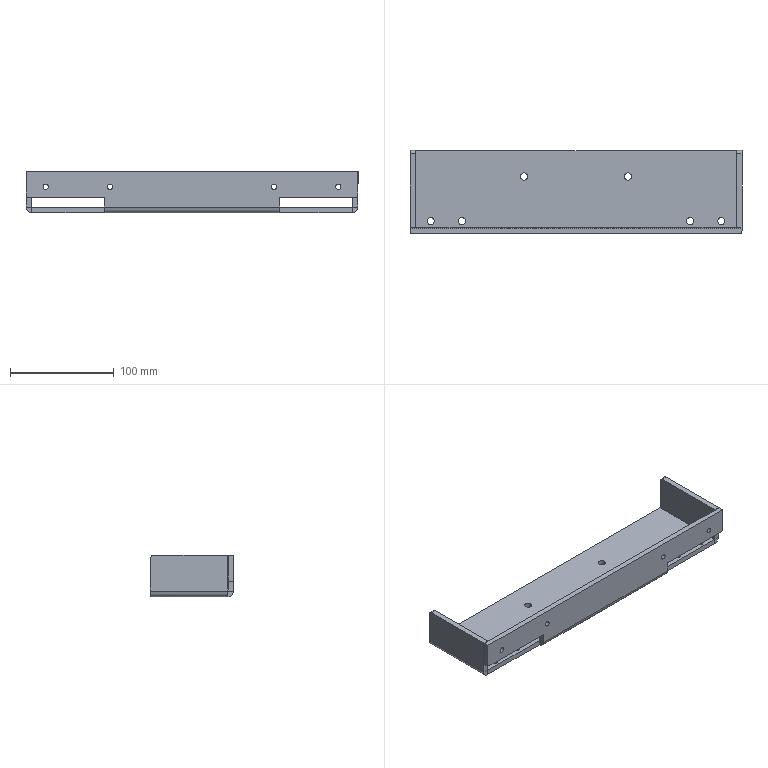Part | SolidWorks | features HoleWzd 3, MoveFace 2, EdgeFlange 1, Fillet 1, FlatPattern 1, ICE 1, MirrorPattern 1, SMBaseFlange 1, SheetMetal 1 | 1 solid | 62 faces | box 320 x 80 x 40 mm | volume 194537 mm3 | plane 32 | cylinder 28 | spline 2 | commonest cylinder face diameters 7 x12 5 x8 1 x3 11 x3 6 x2